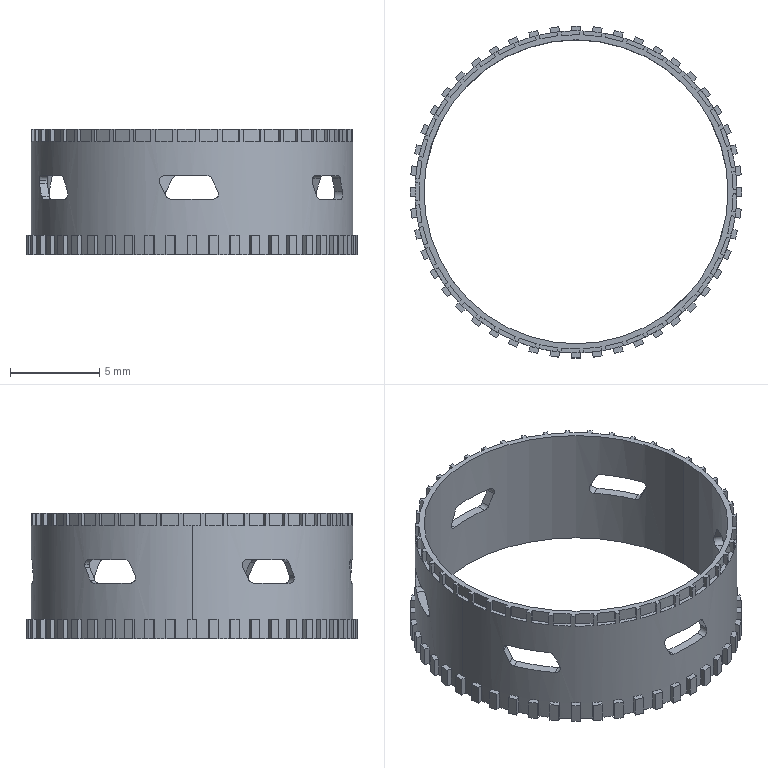Part | SolidWorks | features ICE 4, CirPattern 3, Extrusion 1 | 1 solid | 431 faces | box 18.565 x 18.565 x 7 mm | volume 181.204 mm3 | plane 398 | cylinder 33 | commonest cylinder face diameters 0.6 x29 17 x2 18 x2